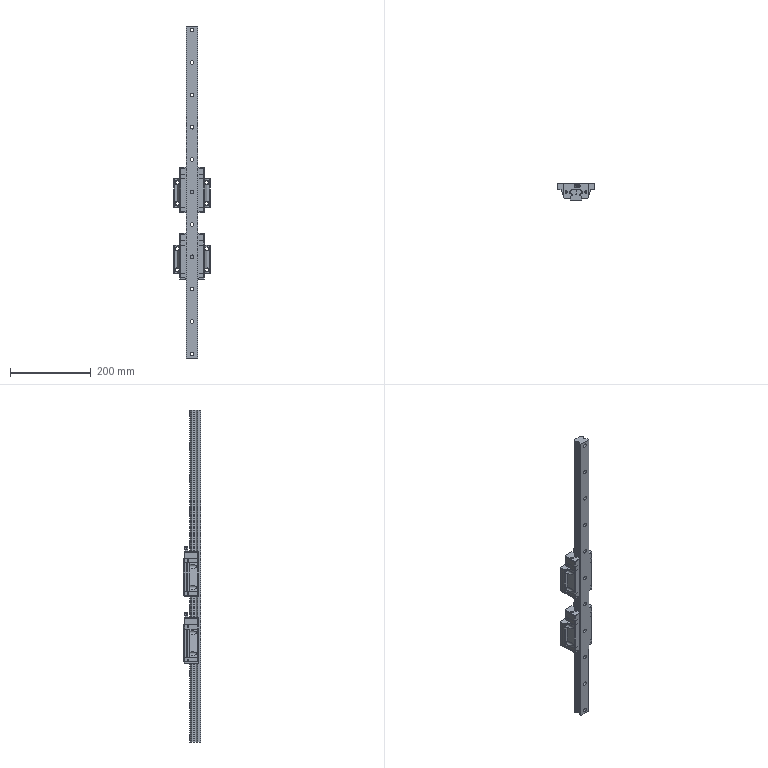Part | SolidWorks | features LocalLPattern 1, ReferencePattern 1 | 15 solids | 1031 faces | box 90 x 42 x 820 mm | volume 939194 mm3 | plane 677 | cylinder 238 | torus 50 | cone 46 | sphere 20 | commonest cylinder face diameters 2.822 x78 9 x38 4.26 x24 14 x22 0.575 x16 4.788 x16